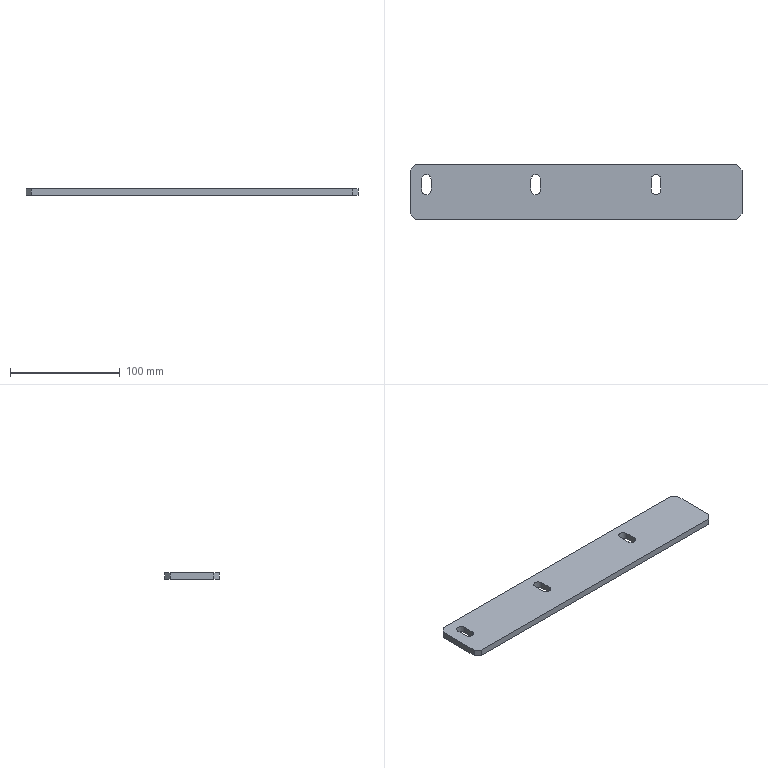Part | STEP file | 1_id1518_x_t | 1 solid | 22 faces | box 303 x 50 x 6 mm | volume 88049 mm3 | plane 16 | cylinder 6 | commonest cylinder face diameters 8.5 x6